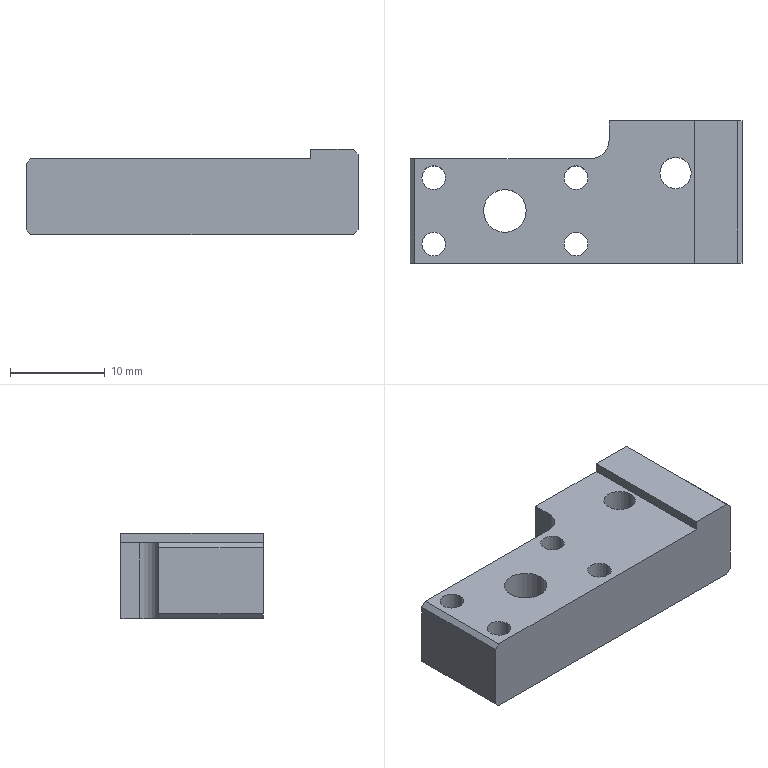Part | STEP file | FBDS-CS-035 | 1 solid | 30 faces | box 35 x 15 x 9 mm | volume 3093 mm3 | cylinder 15 | plane 15 | commonest cylinder face diameters 2.5 x8 3.3 x2 4.5 x2 8 x2 4 x1
STEP:
#1=CARTESIAN_POINT('',(26.35,-1.5,8.));
#2=VERTEX_POINT('',#1);
#3=CARTESIAN_POINT('',(29.65,-1.5,8.));
#4=VERTEX_POINT('',#3);
#5=CARTESIAN_POINT('',(28.,-1.5,8.));
#6=DIRECTION('',(0.,0.,1.));
#7=DIRECTION('',(1.,0.,0.));
#8=AXIS2_PLACEMENT_3D('',#5,#6,#7);
#9=CIRCLE('',#8,1.65);
#10=EDGE_CURVE('',#2,#4,#9,.T.);
#11=ORIENTED_EDGE('',*,*,#10,.T.);
#12=CARTESIAN_POINT('',(29.65,-1.5,0.));
#13=VERTEX_POINT('',#12);
#14=CARTESIAN_POINT('',(29.65,-1.5,0.));
#15=DIRECTION('',(0.,0.,-1.));
#16=VECTOR('',#15,1000.);
#17=LINE('',#14,#16);
#18=EDGE_CURVE('',#4,#13,#17,.T.);
#19=ORIENTED_EDGE('',*,*,#18,.T.);
#20=CARTESIAN_POINT('',(26.35,-1.5,0.));
#21=VERTEX_POINT('',#20);
#22=CARTESIAN_POINT('',(28.,-1.5,0.));
#23=DIRECTION('',(0.,0.,-1.));
#24=DIRECTION('',(-1.,0.,0.));
#25=AXIS2_PLACEMENT_3D('',#22,#23,#24);
#26=CIRCLE('',#25,1.65);
#27=EDGE_CURVE('',#13,#21,#26,.T.);
#28=ORIENTED_EDGE('',*,*,#27,.T.);
#29=CARTESIAN_POINT('',(26.35,-1.5,0.));
#30=DIRECTION('',(0.,0.,-1.));
#31=VECTOR('',#30,1000.);
#32=LINE('',#29,#31);
#33=EDGE_CURVE('',#2,#21,#32,.T.);
#34=ORIENTED_EDGE('',*,*,#33,.F.);
#35=EDGE_LOOP('',(#11,#19,#28,#34));
#36=FACE_OUTER_BOUND('',#35,.T.);
#37=CARTESIAN_POINT('',(28.,-1.5,0.));
#38=DIRECTION('',(0.,0.,-1.));
#39=DIRECTION('',(-1.,0.,0.));
#40=AXIS2_PLACEMENT_3D('',#37,#38,#39);
#41=CYLINDRICAL_SURFACE('',#40,1.65);
#42=ADVANCED_FACE('',(#36),#41,.F.);
#43=CARTESIAN_POINT('',(14.,-5.5,4.6));
#44=VERTEX_POINT('',#43);
#45=CARTESIAN_POINT('',(6.,-5.5,4.6));
#46=VERTEX_POINT('',#45);
#47=CARTESIAN_POINT('',(10.,-5.5,4.6));
#48=DIRECTION('',(0.,0.,-1.));
#49=DIRECTION('',(-1.,0.,0.));
#50=AXIS2_PLACEMENT_3D('',#47,#48,#49);
#51=CIRCLE('',#50,4.);
#52=EDGE_CURVE('',#44,#46,#51,.T.);
#53=ORIENTED_EDGE('',*,*,#52,.F.);
#54=CARTESIAN_POINT('',(14.,-5.5,0.));
#55=VERTEX_POINT('',#54);
#56=CARTESIAN_POINT('',(14.,-5.5,0.));
#57=DIRECTION('',(0.,0.,-1.));
#58=VECTOR('',#57,1000.);
#59=LINE('',#56,#58);
#60=EDGE_CURVE('',#44,#55,#59,.T.);
#61=ORIENTED_EDGE('',*,*,#60,.T.);
#62=CARTESIAN_POINT('',(6.,-5.5,0.));
#63=VERTEX_POINT('',#62);
#64=CARTESIAN_POINT('',(10.,-5.5,0.));
#65=DIRECTION('',(0.,0.,-1.));
#66=DIRECTION('',(-1.,0.,0.));
#67=AXIS2_PLACEMENT_3D('',#64,#65,#66);
#68=CIRCLE('',#67,4.);
#69=EDGE_CURVE('',#55,#63,#68,.T.);
#70=ORIENTED_EDGE('',*,*,#69,.T.);
#71=CARTESIAN_POINT('',(6.,-5.5,0.));
#72=DIRECTION('',(0.,0.,-1.));
#73=VECTOR('',#72,1000.);
#74=LINE('',#71,#73);
#75=EDGE_CURVE('',#46,#63,#74,.T.);
#76=ORIENTED_EDGE('',*,*,#75,.F.);
#77=EDGE_LOOP('',(#53,#61,#70,#76));
#78=FACE_OUTER_BOUND('',#77,.T.);
#79=CARTESIAN_POINT('',(10.,-5.5,0.));
#80=DIRECTION('',(0.,0.,-1.));
#81=DIRECTION('',(-1.,0.,0.));
#82=AXIS2_PLACEMENT_3D('',#79,#80,#81);
#83=CYLINDRICAL_SURFACE('',#82,4.);
#84=ADVANCED_FACE('',(#78),#83,.F.);
#85=CARTESIAN_POINT('',(7.75,-5.5,8.));
#86=VERTEX_POINT('',#85);
#87=CARTESIAN_POINT('',(12.25,-5.5,8.));
#88=VERTEX_POINT('',#87);
#89=CARTESIAN_POINT('',(10.,-5.5,8.));
#90=DIRECTION('',(0.,0.,1.));
#91=DIRECTION('',(1.,0.,0.));
#92=AXIS2_PLACEMENT_3D('',#89,#90,#91);
#93=CIRCLE('',#92,2.25);
#94=EDGE_CURVE('',#86,#88,#93,.T.);
#95=ORIENTED_EDGE('',*,*,#94,.T.);
#96=CARTESIAN_POINT('',(12.25,-5.5,4.6));
#97=VERTEX_POINT('',#96);
#98=CARTESIAN_POINT('',(12.25,-5.5,0.));
#99=DIRECTION('',(0.,0.,-1.));
#100=VECTOR('',#99,1000.);
#101=LINE('',#98,#100);
#102=EDGE_CURVE('',#88,#97,#101,.T.);
#103=ORIENTED_EDGE('',*,*,#102,.T.);
#104=CARTESIAN_POINT('',(7.75,-5.5,4.6));
#105=VERTEX_POINT('',#104);
#106=CARTESIAN_POINT('',(10.,-5.5,4.6));
#107=DIRECTION('',(0.,0.,-1.));
#108=DIRECTION('',(-1.,0.,0.));
#109=AXIS2_PLACEMENT_3D('',#106,#107,#108);
#110=CIRCLE('',#109,2.25);
#111=EDGE_CURVE('',#97,#105,#110,.T.);
#112=ORIENTED_EDGE('',*,*,#111,.T.);
#113=CARTESIAN_POINT('',(7.75,-5.5,0.));
#114=DIRECTION('',(0.,0.,-1.));
#115=VECTOR('',#114,1000.);
#116=LINE('',#113,#115);
#117=EDGE_CURVE('',#86,#105,#116,.T.);
#118=ORIENTED_EDGE('',*,*,#117,.F.);
#119=EDGE_LOOP('',(#95,#103,#112,#118));
#120=FACE_OUTER_BOUND('',#119,.T.);
#121=CARTESIAN_POINT('',(10.,-5.5,0.));
#122=DIRECTION('',(0.,0.,-1.));
#123=DIRECTION('',(-1.,0.,0.));
#124=AXIS2_PLACEMENT_3D('',#121,#122,#123);
#125=CYLINDRICAL_SURFACE('',#124,2.25);
#126=ADVANCED_FACE('',(#120),#125,.F.);
#127=CARTESIAN_POINT('',(16.25,-2.,8.));
#128=VERTEX_POINT('',#127);
#129=CARTESIAN_POINT('',(18.75,-2.,8.));
#130=VERTEX_POINT('',#129);
#131=CARTESIAN_POINT('',(17.5,-2.,8.));
#132=DIRECTION('',(0.,0.,1.));
#133=DIRECTION('',(1.,0.,0.));
#134=AXIS2_PLACEMENT_3D('',#131,#132,#133);
#135=CIRCLE('',#134,1.25);
#136=EDGE_CURVE('',#128,#130,#135,.T.);
#137=ORIENTED_EDGE('',*,*,#136,.T.);
#138=CARTESIAN_POINT('',(18.75,-2.,0.));
#139=VERTEX_POINT('',#138);
#140=CARTESIAN_POINT('',(18.75,-2.,0.));
#141=DIRECTION('',(0.,0.,-1.));
#142=VECTOR('',#141,1000.);
#143=LINE('',#140,#142);
#144=EDGE_CURVE('',#130,#139,#143,.T.);
#145=ORIENTED_EDGE('',*,*,#144,.T.);
#146=CARTESIAN_POINT('',(16.25,-2.,0.));
#147=VERTEX_POINT('',#146);
#148=CARTESIAN_POINT('',(17.5,-2.,0.));
#149=DIRECTION('',(0.,0.,-1.));
#150=DIRECTION('',(-1.,0.,0.));
#151=AXIS2_PLACEMENT_3D('',#148,#149,#150);
#152=CIRCLE('',#151,1.25);
#153=EDGE_CURVE('',#139,#147,#152,.T.);
#154=ORIENTED_EDGE('',*,*,#153,.T.);
#155=CARTESIAN_POINT('',(16.25,-2.,0.));
#156=DIRECTION('',(0.,0.,-1.));
#157=VECTOR('',#156,1000.);
#158=LINE('',#155,#157);
#159=EDGE_CURVE('',#128,#147,#158,.T.);
#160=ORIENTED_EDGE('',*,*,#159,.F.);
#161=EDGE_LOOP('',(#137,#145,#154,#160));
#162=FACE_OUTER_BOUND('',#161,.T.);
#163=CARTESIAN_POINT('',(17.5,-2.,0.));
#164=DIRECTION('',(0.,0.,-1.));
#165=DIRECTION('',(-1.,0.,0.));
#166=AXIS2_PLACEMENT_3D('',#163,#164,#165);
#167=CYLINDRICAL_SURFACE('',#166,1.25);
#168=ADVANCED_FACE('',(#162),#167,.F.);
#169=CARTESIAN_POINT('',(16.25,-9.,8.));
#170=VERTEX_POINT('',#169);
#171=CARTESIAN_POINT('',(18.75,-9.,8.));
#172=VERTEX_POINT('',#171);
#173=CARTESIAN_POINT('',(17.5,-9.,8.));
#174=DIRECTION('',(0.,0.,1.));
#175=DIRECTION('',(1.,0.,0.));
#176=AXIS2_PLACEMENT_3D('',#173,#174,#175);
#177=CIRCLE('',#176,1.25);
#178=EDGE_CURVE('',#170,#172,#177,.T.);
#179=ORIENTED_EDGE('',*,*,#178,.T.);
#180=CARTESIAN_POINT('',(18.75,-9.,0.));
#181=VERTEX_POINT('',#180);
#182=CARTESIAN_POINT('',(18.75,-9.,0.));
#183=DIRECTION('',(0.,0.,-1.));
#184=VECTOR('',#183,1000.);
#185=LINE('',#182,#184);
#186=EDGE_CURVE('',#172,#181,#185,.T.);
#187=ORIENTED_EDGE('',*,*,#186,.T.);
#188=CARTESIAN_POINT('',(16.25,-9.,0.));
#189=VERTEX_POINT('',#188);
#190=CARTESIAN_POINT('',(17.5,-9.,0.));
#191=DIRECTION('',(0.,0.,-1.));
#192=DIRECTION('',(-1.,0.,0.));
#193=AXIS2_PLACEMENT_3D('',#190,#191,#192);
#194=CIRCLE('',#193,1.25);
#195=EDGE_CURVE('',#181,#189,#194,.T.);
#196=ORIENTED_EDGE('',*,*,#195,.T.);
#197=CARTESIAN_POINT('',(16.25,-9.,0.));
#198=DIRECTION('',(0.,0.,-1.));
#199=VECTOR('',#198,1000.);
#200=LINE('',#197,#199);
#201=EDGE_CURVE('',#170,#189,#200,.T.);
#202=ORIENTED_EDGE('',*,*,#201,.F.);
#203=EDGE_LOOP('',(#179,#187,#196,#202));
#204=FACE_OUTER_BOUND('',#203,.T.);
#205=CARTESIAN_POINT('',(17.5,-9.,0.));
#206=DIRECTION('',(0.,0.,-1.));
#207=DIRECTION('',(-1.,0.,0.));
#208=AXIS2_PLACEMENT_3D('',#205,#206,#207);
#209=CYLINDRICAL_SURFACE('',#208,1.25);
#210=ADVANCED_FACE('',(#204),#209,.F.);
#211=CARTESIAN_POINT('',(1.25,-9.,8.));
#212=VERTEX_POINT('',#211);
#213=CARTESIAN_POINT('',(3.75,-9.,8.));
#214=VERTEX_POINT('',#213);
#215=CARTESIAN_POINT('',(2.5,-9.,8.));
#216=DIRECTION('',(0.,0.,1.));
#217=DIRECTION('',(1.,0.,0.));
#218=AXIS2_PLACEMENT_3D('',#215,#216,#217);
#219=CIRCLE('',#218,1.25);
#220=EDGE_CURVE('',#212,#214,#219,.T.);
#221=ORIENTED_EDGE('',*,*,#220,.T.);
#222=CARTESIAN_POINT('',(3.75,-9.,0.));
#223=VERTEX_POINT('',#222);
#224=CARTESIAN_POINT('',(3.75,-9.,0.));
#225=DIRECTION('',(0.,0.,-1.));
#226=VECTOR('',#225,1000.);
#227=LINE('',#224,#226);
#228=EDGE_CURVE('',#214,#223,#227,.T.);
#229=ORIENTED_EDGE('',*,*,#228,.T.);
#230=CARTESIAN_POINT('',(1.25,-9.,0.));
#231=VERTEX_POINT('',#230);
#232=CARTESIAN_POINT('',(2.5,-9.,0.));
#233=DIRECTION('',(0.,0.,-1.));
#234=DIRECTION('',(-1.,0.,0.));
#235=AXIS2_PLACEMENT_3D('',#232,#233,#234);
#236=CIRCLE('',#235,1.25);
#237=EDGE_CURVE('',#223,#231,#236,.T.);
#238=ORIENTED_EDGE('',*,*,#237,.T.);
#239=CARTESIAN_POINT('',(1.25,-9.,0.));
#240=DIRECTION('',(0.,0.,-1.));
#241=VECTOR('',#240,1000.);
#242=LINE('',#239,#241);
#243=EDGE_CURVE('',#212,#231,#242,.T.);
#244=ORIENTED_EDGE('',*,*,#243,.F.);
#245=EDGE_LOOP('',(#221,#229,#238,#244));
#246=FACE_OUTER_BOUND('',#245,.T.);
#247=CARTESIAN_POINT('',(2.5,-9.,0.));
#248=DIRECTION('',(0.,0.,-1.));
#249=DIRECTION('',(-1.,0.,0.));
#250=AXIS2_PLACEMENT_3D('',#247,#248,#249);
#251=CYLINDRICAL_SURFACE('',#250,1.25);
#252=ADVANCED_FACE('',(#246),#251,.F.);
#253=CARTESIAN_POINT('',(1.25,-2.,8.));
#254=VERTEX_POINT('',#253);
#255=CARTESIAN_POINT('',(3.75,-2.,8.));
#256=VERTEX_POINT('',#255);
#257=CARTESIAN_POINT('',(2.5,-2.,8.));
#258=DIRECTION('',(0.,0.,1.));
#259=DIRECTION('',(1.,0.,0.));
#260=AXIS2_PLACEMENT_3D('',#257,#258,#259);
#261=CIRCLE('',#260,1.25);
#262=EDGE_CURVE('',#254,#256,#261,.T.);
#263=ORIENTED_EDGE('',*,*,#262,.T.);
#264=CARTESIAN_POINT('',(3.75,-2.,0.));
#265=VERTEX_POINT('',#264);
#266=CARTESIAN_POINT('',(3.75,-2.,0.));
#267=DIRECTION('',(0.,0.,-1.));
#268=VECTOR('',#267,1000.);
#269=LINE('',#266,#268);
#270=EDGE_CURVE('',#256,#265,#269,.T.);
#271=ORIENTED_EDGE('',*,*,#270,.T.);
#272=CARTESIAN_POINT('',(1.25,-2.,0.));
#273=VERTEX_POINT('',#272);
#274=CARTESIAN_POINT('',(2.5,-2.,0.));
#275=DIRECTION('',(0.,0.,-1.));
#276=DIRECTION('',(-1.,0.,0.));
#277=AXIS2_PLACEMENT_3D('',#274,#275,#276);
#278=CIRCLE('',#277,1.25);
#279=EDGE_CURVE('',#265,#273,#278,.T.);
#280=ORIENTED_EDGE('',*,*,#279,.T.);
#281=CARTESIAN_POINT('',(1.25,-2.,0.));
#282=DIRECTION('',(0.,0.,-1.));
#283=VECTOR('',#282,1000.);
#284=LINE('',#281,#283);
#285=EDGE_CURVE('',#254,#273,#284,.T.);
#286=ORIENTED_EDGE('',*,*,#285,.F.);
#287=EDGE_LOOP('',(#263,#271,#280,#286));
#288=FACE_OUTER_BOUND('',#287,.T.);
#289=CARTESIAN_POINT('',(2.5,-2.,0.));
#290=DIRECTION('',(0.,0.,-1.));
#291=DIRECTION('',(-1.,0.,0.));
#292=AXIS2_PLACEMENT_3D('',#289,#290,#291);
#293=CYLINDRICAL_SURFACE('',#292,1.25);
#294=ADVANCED_FACE('',(#288),#293,.F.);
#295=CARTESIAN_POINT('',(19.,0.,8.));
#296=VERTEX_POINT('',#295);
#297=CARTESIAN_POINT('',(0.5,0.,8.));
#298=VERTEX_POINT('',#297);
#299=CARTESIAN_POINT('',(0.,0.,8.));
#300=DIRECTION('',(-1.,0.,0.));
#301=VECTOR('',#300,1000.);
#302=LINE('',#299,#301);
#303=EDGE_CURVE('',#296,#298,#302,.T.);
#304=ORIENTED_EDGE('',*,*,#303,.F.);
#305=CARTESIAN_POINT('',(19.,0.,0.));
#306=VERTEX_POINT('',#305);
#307=CARTESIAN_POINT('',(19.,0.,0.));
#308=DIRECTION('',(0.,0.,-1.));
#309=VECTOR('',#308,1000.);
#310=LINE('',#307,#309);
#311=EDGE_CURVE('',#296,#306,#310,.T.);
#312=ORIENTED_EDGE('',*,*,#311,.T.);
#313=CARTESIAN_POINT('',(0.5,0.,0.));
#314=VERTEX_POINT('',#313);
#315=CARTESIAN_POINT('',(0.,0.,0.));
#316=DIRECTION('',(-1.,0.,0.));
#317=VECTOR('',#316,1000.);
#318=LINE('',#315,#317);
#319=EDGE_CURVE('',#306,#314,#318,.T.);
#320=ORIENTED_EDGE('',*,*,#319,.T.);
#321=CARTESIAN_POINT('',(0.,0.,0.5));
#322=VERTEX_POINT('',#321);
#323=CARTESIAN_POINT('',(0.,0.,0.5));
#324=DIRECTION('',(-0.7071,0.,0.7071));
#325=VECTOR('',#324,1000.);
#326=LINE('',#323,#325);
#327=EDGE_CURVE('',#314,#322,#326,.T.);
#328=ORIENTED_EDGE('',*,*,#327,.T.);
#329=CARTESIAN_POINT('',(0.,0.,7.5));
#330=VERTEX_POINT('',#329);
#331=CARTESIAN_POINT('',(0.,0.,8.));
#332=DIRECTION('',(0.,0.,-1.));
#333=VECTOR('',#332,1000.);
#334=LINE('',#331,#333);
#335=EDGE_CURVE('',#330,#322,#334,.T.);
#336=ORIENTED_EDGE('',*,*,#335,.F.);
#337=CARTESIAN_POINT('',(0.5,0.,8.));
#338=DIRECTION('',(0.7071,0.,0.7071));
#339=VECTOR('',#338,1000.);
#340=LINE('',#337,#339);
#341=EDGE_CURVE('',#330,#298,#340,.T.);
#342=ORIENTED_EDGE('',*,*,#341,.T.);
#343=EDGE_LOOP('',(#304,#312,#320,#328,#336,#342));
#344=FACE_OUTER_BOUND('',#343,.T.);
#345=CARTESIAN_POINT('',(0.,0.,8.));
#346=DIRECTION('',(0.,-1.,0.));
#347=DIRECTION('',(0.,0.,-1.));
#348=AXIS2_PLACEMENT_3D('',#345,#346,#347);
#349=PLANE('',#348);
#350=ADVANCED_FACE('',(#344),#349,.F.);
#351=ORIENTED_EDGE('',*,*,#335,.T.);
#352=CARTESIAN_POINT('',(0.,-11.,0.5));
#353=VERTEX_POINT('',#352);
#354=CARTESIAN_POINT('',(0.,0.,0.5));
#355=DIRECTION('',(0.,-1.,0.));
#356=VECTOR('',#355,1000.);
#357=LINE('',#354,#356);
#358=EDGE_CURVE('',#322,#353,#357,.T.);
#359=ORIENTED_EDGE('',*,*,#358,.T.);
#360=CARTESIAN_POINT('',(0.,-11.,7.5));
#361=VERTEX_POINT('',#360);
#362=CARTESIAN_POINT('',(0.,-11.,8.));
#363=DIRECTION('',(0.,0.,-1.));
#364=VECTOR('',#363,1000.);
#365=LINE('',#362,#364);
#366=EDGE_CURVE('',#361,#353,#365,.T.);
#367=ORIENTED_EDGE('',*,*,#366,.F.);
#368=CARTESIAN_POINT('',(0.,0.,7.5));
#369=DIRECTION('',(0.,1.,0.));
#370=VECTOR('',#369,1000.);
#371=LINE('',#368,#370);
#372=EDGE_CURVE('',#361,#330,#371,.T.);
#373=ORIENTED_EDGE('',*,*,#372,.T.);
#374=EDGE_LOOP('',(#351,#359,#367,#373));
#375=FACE_OUTER_BOUND('',#374,.T.);
#376=CARTESIAN_POINT('',(0.,0.,8.));
#377=DIRECTION('',(1.,0.,0.));
#378=DIRECTION('',(0.,0.,-1.));
#379=AXIS2_PLACEMENT_3D('',#376,#377,#378);
#380=PLANE('',#379);
#381=ADVANCED_FACE('',(#375),#380,.F.);
#382=CARTESIAN_POINT('',(35.,-11.,8.5));
#383=VERTEX_POINT('',#382);
#384=CARTESIAN_POINT('',(35.,-11.,0.5));
#385=VERTEX_POINT('',#384);
#386=CARTESIAN_POINT('',(35.,-11.,8.));
#387=DIRECTION('',(0.,0.,-1.));
#388=VECTOR('',#387,1000.);
#389=LINE('',#386,#388);
#390=EDGE_CURVE('',#383,#385,#389,.T.);
#391=ORIENTED_EDGE('',*,*,#390,.F.);
#392=CARTESIAN_POINT('',(34.5,-11.,9.));
#393=VERTEX_POINT('',#392);
#394=CARTESIAN_POINT('',(34.5,-11.,9.));
#395=DIRECTION('',(-0.7071,0.,0.7071));
#396=VECTOR('',#395,1000.);
#397=LINE('',#394,#396);
#398=EDGE_CURVE('',#383,#393,#397,.T.);
#399=ORIENTED_EDGE('',*,*,#398,.T.);
#400=CARTESIAN_POINT('',(30.,-11.,9.));
#401=VERTEX_POINT('',#400);
#402=CARTESIAN_POINT('',(35.,-11.,9.));
#403=DIRECTION('',(1.,0.,0.));
#404=VECTOR('',#403,1000.);
#405=LINE('',#402,#404);
#406=EDGE_CURVE('',#401,#393,#405,.T.);
#407=ORIENTED_EDGE('',*,*,#406,.F.);
#408=CARTESIAN_POINT('',(30.,-11.,8.));
#409=VERTEX_POINT('',#408);
#410=CARTESIAN_POINT('',(30.,-11.,9.));
#411=DIRECTION('',(0.,0.,-1.));
#412=VECTOR('',#411,1000.);
#413=LINE('',#410,#412);
#414=EDGE_CURVE('',#401,#409,#413,.T.);
#415=ORIENTED_EDGE('',*,*,#414,.T.);
#416=CARTESIAN_POINT('',(0.5,-11.,8.));
#417=VERTEX_POINT('',#416);
#418=CARTESIAN_POINT('',(0.,-11.,8.));
#419=DIRECTION('',(1.,0.,0.));
#420=VECTOR('',#419,1000.);
#421=LINE('',#418,#420);
#422=EDGE_CURVE('',#417,#409,#421,.T.);
#423=ORIENTED_EDGE('',*,*,#422,.F.);
#424=CARTESIAN_POINT('',(0.5,-11.,8.));
#425=DIRECTION('',(-0.7071,0.,-0.7071));
#426=VECTOR('',#425,1000.);
#427=LINE('',#424,#426);
#428=EDGE_CURVE('',#417,#361,#427,.T.);
#429=ORIENTED_EDGE('',*,*,#428,.T.);
#430=ORIENTED_EDGE('',*,*,#366,.T.);
#431=CARTESIAN_POINT('',(0.5,-11.,0.));
#432=VERTEX_POINT('',#431);
#433=CARTESIAN_POINT('',(0.,-11.,0.5));
#434=DIRECTION('',(0.7071,0.,-0.7071));
#435=VECTOR('',#434,1000.);
#436=LINE('',#433,#435);
#437=EDGE_CURVE('',#353,#432,#436,.T.);
#438=ORIENTED_EDGE('',*,*,#437,.T.);
#439=CARTESIAN_POINT('',(34.5,-11.,0.));
#440=VERTEX_POINT('',#439);
#441=CARTESIAN_POINT('',(0.,-11.,0.));
#442=DIRECTION('',(1.,0.,0.));
#443=VECTOR('',#442,1000.);
#444=LINE('',#441,#443);
#445=EDGE_CURVE('',#432,#440,#444,.T.);
#446=ORIENTED_EDGE('',*,*,#445,.T.);
#447=CARTESIAN_POINT('',(35.,-11.,0.5));
#448=DIRECTION('',(0.7071,0.,0.7071));
#449=VECTOR('',#448,1000.);
#450=LINE('',#447,#449);
#451=EDGE_CURVE('',#440,#385,#450,.T.);
#452=ORIENTED_EDGE('',*,*,#451,.T.);
#453=EDGE_LOOP('',(#391,#399,#407,#415,#423,#429,#430,#438,#446,#452));
#454=FACE_OUTER_BOUND('',#453,.T.);
#455=CARTESIAN_POINT('',(0.,-11.,8.));
#456=DIRECTION('',(0.,1.,0.));
#457=DIRECTION('',(0.,0.,1.));
#458=AXIS2_PLACEMENT_3D('',#455,#456,#457);
#459=PLANE('',#458);
#460=ADVANCED_FACE('',(#454),#459,.F.);
#461=CARTESIAN_POINT('',(35.,4.,0.5));
#462=VERTEX_POINT('',#461);
#463=CARTESIAN_POINT('',(35.,0.,0.5));
#464=DIRECTION('',(0.,1.,0.));
#465=VECTOR('',#464,1000.);
#466=LINE('',#463,#465);
#467=EDGE_CURVE('',#385,#462,#466,.T.);
#468=ORIENTED_EDGE('',*,*,#467,.T.);
#469=CARTESIAN_POINT('',(35.,4.,8.5));
#470=VERTEX_POINT('',#469);
#471=CARTESIAN_POINT('',(35.,4.,8.5));
#472=DIRECTION('',(0.,0.,-1.));
#473=VECTOR('',#472,1000.);
#474=LINE('',#471,#473);
#475=EDGE_CURVE('',#470,#462,#474,.T.);
#476=ORIENTED_EDGE('',*,*,#475,.F.);
#477=CARTESIAN_POINT('',(35.,0.,8.5));
#478=DIRECTION('',(0.,-1.,0.));
#479=VECTOR('',#478,1000.);
#480=LINE('',#477,#479);
#481=EDGE_CURVE('',#470,#383,#480,.T.);
#482=ORIENTED_EDGE('',*,*,#481,.T.);
#483=ORIENTED_EDGE('',*,*,#390,.T.);
#484=EDGE_LOOP('',(#468,#476,#482,#483));
#485=FACE_OUTER_BOUND('',#484,.T.);
#486=CARTESIAN_POINT('',(35.,0.,8.));
#487=DIRECTION('',(-1.,0.,0.));
#488=DIRECTION('',(0.,0.,1.));
#489=AXIS2_PLACEMENT_3D('',#486,#487,#488);
#490=PLANE('',#489);
#491=ADVANCED_FACE('',(#485),#490,.F.);
#492=ORIENTED_EDGE('',*,*,#10,.F.);
#493=CARTESIAN_POINT('',(28.,-1.5,8.));
#494=DIRECTION('',(0.,0.,1.));
#495=DIRECTION('',(1.,0.,0.));
#496=AXIS2_PLACEMENT_3D('',#493,#494,#495);
#497=CIRCLE('',#496,1.65);
#498=EDGE_CURVE('',#4,#2,#497,.T.);
#499=ORIENTED_EDGE('',*,*,#498,.F.);
#500=EDGE_LOOP('',(#492,#499));
#501=FACE_BOUND('',#500,.T.);
#502=CARTESIAN_POINT('',(30.,4.,8.));
#503=VERTEX_POINT('',#502);
#504=CARTESIAN_POINT('',(30.,0.,8.));
#505=DIRECTION('',(0.,-1.,0.));
#506=VECTOR('',#505,1000.);
#507=LINE('',#504,#506);
#508=EDGE_CURVE('',#503,#409,#507,.T.);
#509=ORIENTED_EDGE('',*,*,#508,.F.);
#510=CARTESIAN_POINT('',(21.,4.,8.));
#511=VERTEX_POINT('',#510);
#512=CARTESIAN_POINT('',(21.,4.,8.));
#513=DIRECTION('',(1.,0.,0.));
#514=VECTOR('',#513,1000.);
#515=LINE('',#512,#514);
#516=EDGE_CURVE('',#511,#503,#515,.T.);
#517=ORIENTED_EDGE('',*,*,#516,.F.);
#518=CARTESIAN_POINT('',(21.,2.,8.));
#519=VERTEX_POINT('',#518);
#520=CARTESIAN_POINT('',(21.,4.,8.));
#521=DIRECTION('',(0.,-1.,0.));
#522=VECTOR('',#521,1000.);
#523=LINE('',#520,#522);
#524=EDGE_CURVE('',#511,#519,#523,.T.);
#525=ORIENTED_EDGE('',*,*,#524,.T.);
#526=CARTESIAN_POINT('',(19.,2.,8.));
#527=DIRECTION('',(0.,0.,-1.));
#528=DIRECTION('',(1.,0.,0.));
#529=AXIS2_PLACEMENT_3D('',#526,#527,#528);
#530=CIRCLE('',#529,2.);
#531=EDGE_CURVE('',#519,#296,#530,.T.);
#532=ORIENTED_EDGE('',*,*,#531,.T.);
#533=ORIENTED_EDGE('',*,*,#303,.T.);
#534=CARTESIAN_POINT('',(0.5,-11.,8.));
#535=DIRECTION('',(0.,-1.,0.));
#536=VECTOR('',#535,1000.);
#537=LINE('',#534,#536);
#538=EDGE_CURVE('',#298,#417,#537,.T.);
#539=ORIENTED_EDGE('',*,*,#538,.T.);
#540=ORIENTED_EDGE('',*,*,#422,.T.);
#541=EDGE_LOOP('',(#509,#517,#525,#532,#533,#539,#540));
#542=FACE_OUTER_BOUND('',#541,.T.);
#543=ORIENTED_EDGE('',*,*,#94,.F.);
#544=CARTESIAN_POINT('',(10.,-5.5,8.));
#545=DIRECTION('',(0.,0.,1.));
#546=DIRECTION('',(1.,0.,0.));
#547=AXIS2_PLACEMENT_3D('',#544,#545,#546);
#548=CIRCLE('',#547,2.25);
#549=EDGE_CURVE('',#88,#86,#548,.T.);
#550=ORIENTED_EDGE('',*,*,#549,.F.);
#551=EDGE_LOOP('',(#543,#550));
#552=FACE_BOUND('',#551,.T.);
#553=ORIENTED_EDGE('',*,*,#136,.F.);
#554=CARTESIAN_POINT('',(17.5,-2.,8.));
#555=DIRECTION('',(0.,0.,1.));
#556=DIRECTION('',(1.,0.,0.));
#557=AXIS2_PLACEMENT_3D('',#554,#555,#556);
#558=CIRCLE('',#557,1.25);
#559=EDGE_CURVE('',#130,#128,#558,.T.);
#560=ORIENTED_EDGE('',*,*,#559,.F.);
#561=EDGE_LOOP('',(#553,#560));
#562=FACE_BOUND('',#561,.T.);
#563=ORIENTED_EDGE('',*,*,#178,.F.);
#564=CARTESIAN_POINT('',(17.5,-9.,8.));
#565=DIRECTION('',(0.,0.,1.));
#566=DIRECTION('',(1.,0.,0.));
#567=AXIS2_PLACEMENT_3D('',#564,#565,#566);
#568=CIRCLE('',#567,1.25);
#569=EDGE_CURVE('',#172,#170,#568,.T.);
#570=ORIENTED_EDGE('',*,*,#569,.F.);
#571=EDGE_LOOP('',(#563,#570));
#572=FACE_BOUND('',#571,.T.);
#573=ORIENTED_EDGE('',*,*,#220,.F.);
#574=CARTESIAN_POINT('',(2.5,-9.,8.));
#575=DIRECTION('',(0.,0.,1.));
#576=DIRECTION('',(1.,0.,0.));
#577=AXIS2_PLACEMENT_3D('',#574,#575,#576);
#578=CIRCLE('',#577,1.25);
#579=EDGE_CURVE('',#214,#212,#578,.T.);
#580=ORIENTED_EDGE('',*,*,#579,.F.);
#581=EDGE_LOOP('',(#573,#580));
#582=FACE_BOUND('',#581,.T.);
#583=ORIENTED_EDGE('',*,*,#262,.F.);
#584=CARTESIAN_POINT('',(2.5,-2.,8.));
#585=DIRECTION('',(0.,0.,1.));
#586=DIRECTION('',(1.,0.,0.));
#587=AXIS2_PLACEMENT_3D('',#584,#585,#586);
#588=CIRCLE('',#587,1.25);
#589=EDGE_CURVE('',#256,#254,#588,.T.);
#590=ORIENTED_EDGE('',*,*,#589,.F.);
#591=EDGE_LOOP('',(#583,#590));
#592=FACE_BOUND('',#591,.T.);
#593=CARTESIAN_POINT('',(0.,0.,8.));
#594=DIRECTION('',(0.,0.,1.));
#595=DIRECTION('',(1.,0.,0.));
#596=AXIS2_PLACEMENT_3D('',#593,#594,#595);
#597=PLANE('',#596);
#598=ADVANCED_FACE('',(#501,#542,#552,#562,#572,#582,#592),#597,.T.);
#599=CARTESIAN_POINT('',(28.,-1.5,0.));
#600=DIRECTION('',(0.,0.,-1.));
#601=DIRECTION('',(-1.,0.,0.));
#602=AXIS2_PLACEMENT_3D('',#599,#600,#601);
#603=CIRCLE('',#602,1.65);
#604=EDGE_CURVE('',#21,#13,#603,.T.);
#605=ORIENTED_EDGE('',*,*,#604,.F.);
#606=ORIENTED_EDGE('',*,*,#27,.F.);
#607=EDGE_LOOP('',(#605,#606));
#608=FACE_BOUND('',#607,.T.);
#609=CARTESIAN_POINT('',(10.,-5.5,0.));
#610=DIRECTION('',(0.,0.,-1.));
#611=DIRECTION('',(-1.,0.,0.));
#612=AXIS2_PLACEMENT_3D('',#609,#610,#611);
#613=CIRCLE('',#612,4.);
#614=EDGE_CURVE('',#63,#55,#613,.T.);
#615=ORIENTED_EDGE('',*,*,#614,.F.);
#616=ORIENTED_EDGE('',*,*,#69,.F.);
#617=EDGE_LOOP('',(#615,#616));
#618=FACE_BOUND('',#617,.T.);
#619=CARTESIAN_POINT('',(17.5,-2.,0.));
#620=DIRECTION('',(0.,0.,-1.));
#621=DIRECTION('',(-1.,0.,0.));
#622=AXIS2_PLACEMENT_3D('',#619,#620,#621);
#623=CIRCLE('',#622,1.25);
#624=EDGE_CURVE('',#147,#139,#623,.T.);
#625=ORIENTED_EDGE('',*,*,#624,.F.);
#626=ORIENTED_EDGE('',*,*,#153,.F.);
#627=EDGE_LOOP('',(#625,#626));
#628=FACE_BOUND('',#627,.T.);
#629=CARTESIAN_POINT('',(17.5,-9.,0.));
#630=DIRECTION('',(0.,0.,-1.));
#631=DIRECTION('',(-1.,0.,0.));
#632=AXIS2_PLACEMENT_3D('',#629,#630,#631);
#633=CIRCLE('',#632,1.25);
#634=EDGE_CURVE('',#189,#181,#633,.T.);
#635=ORIENTED_EDGE('',*,*,#634,.F.);
#636=ORIENTED_EDGE('',*,*,#195,.F.);
#637=EDGE_LOOP('',(#635,#636));
#638=FACE_BOUND('',#637,.T.);
#639=CARTESIAN_POINT('',(2.5,-9.,0.));
#640=DIRECTION('',(0.,0.,-1.));
#641=DIRECTION('',(-1.,0.,0.));
#642=AXIS2_PLACEMENT_3D('',#639,#640,#641);
#643=CIRCLE('',#642,1.25);
#644=EDGE_CURVE('',#231,#223,#643,.T.);
#645=ORIENTED_EDGE('',*,*,#644,.F.);
#646=ORIENTED_EDGE('',*,*,#237,.F.);
#647=EDGE_LOOP('',(#645,#646));
#648=FACE_BOUND('',#647,.T.);
#649=CARTESIAN_POINT('',(2.5,-2.,0.));
#650=DIRECTION('',(0.,0.,-1.));
#651=DIRECTION('',(-1.,0.,0.));
#652=AXIS2_PLACEMENT_3D('',#649,#650,#651);
#653=CIRCLE('',#652,1.25);
#654=EDGE_CURVE('',#273,#265,#653,.T.);
#655=ORIENTED_EDGE('',*,*,#654,.F.);
#656=ORIENTED_EDGE('',*,*,#279,.F.);
#657=EDGE_LOOP('',(#655,#656));
#658=FACE_BOUND('',#657,.T.);
#659=ORIENTED_EDGE('',*,*,#319,.F.);
#660=CARTESIAN_POINT('',(21.,2.,0.));
#661=VERTEX_POINT('',#660);
#662=CARTESIAN_POINT('',(19.,2.,0.));
#663=DIRECTION('',(0.,0.,1.));
#664=DIRECTION('',(1.,0.,0.));
#665=AXIS2_PLACEMENT_3D('',#662,#663,#664);
#666=CIRCLE('',#665,2.);
#667=EDGE_CURVE('',#306,#661,#666,.T.);
#668=ORIENTED_EDGE('',*,*,#667,.T.);
#669=CARTESIAN_POINT('',(21.,4.,0.));
#670=VERTEX_POINT('',#669);
#671=CARTESIAN_POINT('',(21.,4.,0.));
#672=DIRECTION('',(0.,-1.,0.));
#673=VECTOR('',#672,1000.);
#674=LINE('',#671,#673);
#675=EDGE_CURVE('',#670,#661,#674,.T.);
#676=ORIENTED_EDGE('',*,*,#675,.F.);
#677=CARTESIAN_POINT('',(34.5,4.,0.));
#678=VERTEX_POINT('',#677);
#679=CARTESIAN_POINT('',(34.5,4.,0.));
#680=DIRECTION('',(-1.,0.,0.));
#681=VECTOR('',#680,1000.);
#682=LINE('',#679,#681);
#683=EDGE_CURVE('',#678,#670,#682,.T.);
#684=ORIENTED_EDGE('',*,*,#683,.F.);
#685=CARTESIAN_POINT('',(34.5,0.,0.));
#686=DIRECTION('',(0.,-1.,0.));
#687=VECTOR('',#686,1000.);
#688=LINE('',#685,#687);
#689=EDGE_CURVE('',#678,#440,#688,.T.);
#690=ORIENTED_EDGE('',*,*,#689,.T.);
#691=ORIENTED_EDGE('',*,*,#445,.F.);
#692=CARTESIAN_POINT('',(0.5,0.,0.));
#693=DIRECTION('',(0.,1.,0.));
#694=VECTOR('',#693,1000.);
#695=LINE('',#692,#694);
#696=EDGE_CURVE('',#432,#314,#695,.T.);
#697=ORIENTED_EDGE('',*,*,#696,.T.);
#698=EDGE_LOOP('',(#659,#668,#676,#684,#690,#691,#697));
#699=FACE_OUTER_BOUND('',#698,.T.);
#700=CARTESIAN_POINT('',(0.,0.,0.));
#701=DIRECTION('',(0.,0.,1.));
#702=DIRECTION('',(1.,0.,0.));
#703=AXIS2_PLACEMENT_3D('',#700,#701,#702);
#704=PLANE('',#703);
#705=ADVANCED_FACE('',(#608,#618,#628,#638,#648,#658,#699),#704,.F.);
#706=ORIENTED_EDGE('',*,*,#270,.F.);
#707=ORIENTED_EDGE('',*,*,#589,.T.);
#708=ORIENTED_EDGE('',*,*,#285,.T.);
#709=ORIENTED_EDGE('',*,*,#654,.T.);
#710=EDGE_LOOP('',(#706,#707,#708,#709));
#711=FACE_OUTER_BOUND('',#710,.T.);
#712=CARTESIAN_POINT('',(2.5,-2.,0.));
#713=DIRECTION('',(0.,0.,-1.));
#714=DIRECTION('',(-1.,0.,0.));
#715=AXIS2_PLACEMENT_3D('',#712,#713,#714);
#716=CYLINDRICAL_SURFACE('',#715,1.25);
#717=ADVANCED_FACE('',(#711),#716,.F.);
#718=ORIENTED_EDGE('',*,*,#228,.F.);
#719=ORIENTED_EDGE('',*,*,#579,.T.);
#720=ORIENTED_EDGE('',*,*,#243,.T.);
#721=ORIENTED_EDGE('',*,*,#644,.T.);
#722=EDGE_LOOP('',(#718,#719,#720,#721));
#723=FACE_OUTER_BOUND('',#722,.T.);
#724=CARTESIAN_POINT('',(2.5,-9.,0.));
#725=DIRECTION('',(0.,0.,-1.));
#726=DIRECTION('',(-1.,0.,0.));
#727=AXIS2_PLACEMENT_3D('',#724,#725,#726);
#728=CYLINDRICAL_SURFACE('',#727,1.25);
#729=ADVANCED_FACE('',(#723),#728,.F.);
#730=ORIENTED_EDGE('',*,*,#186,.F.);
#731=ORIENTED_EDGE('',*,*,#569,.T.);
#732=ORIENTED_EDGE('',*,*,#201,.T.);
#733=ORIENTED_EDGE('',*,*,#634,.T.);
#734=EDGE_LOOP('',(#730,#731,#732,#733));
#735=FACE_OUTER_BOUND('',#734,.T.);
#736=CARTESIAN_POINT('',(17.5,-9.,0.));
#737=DIRECTION('',(0.,0.,-1.));
#738=DIRECTION('',(-1.,0.,0.));
#739=AXIS2_PLACEMENT_3D('',#736,#737,#738);
#740=CYLINDRICAL_SURFACE('',#739,1.25);
#741=ADVANCED_FACE('',(#735),#740,.F.);
#742=ORIENTED_EDGE('',*,*,#144,.F.);
#743=ORIENTED_EDGE('',*,*,#559,.T.);
#744=ORIENTED_EDGE('',*,*,#159,.T.);
#745=ORIENTED_EDGE('',*,*,#624,.T.);
#746=EDGE_LOOP('',(#742,#743,#744,#745));
#747=FACE_OUTER_BOUND('',#746,.T.);
#748=CARTESIAN_POINT('',(17.5,-2.,0.));
#749=DIRECTION('',(0.,0.,-1.));
#750=DIRECTION('',(-1.,0.,0.));
#751=AXIS2_PLACEMENT_3D('',#748,#749,#750);
#752=CYLINDRICAL_SURFACE('',#751,1.25);
#753=ADVANCED_FACE('',(#747),#752,.F.);
#754=ORIENTED_EDGE('',*,*,#102,.F.);
#755=ORIENTED_EDGE('',*,*,#549,.T.);
#756=ORIENTED_EDGE('',*,*,#117,.T.);
#757=CARTESIAN_POINT('',(10.,-5.5,4.6));
#758=DIRECTION('',(0.,0.,-1.));
#759=DIRECTION('',(-1.,0.,0.));
#760=AXIS2_PLACEMENT_3D('',#757,#758,#759);
#761=CIRCLE('',#760,2.25);
#762=EDGE_CURVE('',#105,#97,#761,.T.);
#763=ORIENTED_EDGE('',*,*,#762,.T.);
#764=EDGE_LOOP('',(#754,#755,#756,#763));
#765=FACE_OUTER_BOUND('',#764,.T.);
#766=CARTESIAN_POINT('',(10.,-5.5,0.));
#767=DIRECTION('',(0.,0.,-1.));
#768=DIRECTION('',(-1.,0.,0.));
#769=AXIS2_PLACEMENT_3D('',#766,#767,#768);
#770=CYLINDRICAL_SURFACE('',#769,2.25);
#771=ADVANCED_FACE('',(#765),#770,.F.);
#772=ORIENTED_EDGE('',*,*,#762,.F.);
#773=ORIENTED_EDGE('',*,*,#111,.F.);
#774=EDGE_LOOP('',(#772,#773));
#775=FACE_BOUND('',#774,.T.);
#776=CARTESIAN_POINT('',(10.,-5.5,4.6));
#777=DIRECTION('',(0.,0.,-1.));
#778=DIRECTION('',(-1.,0.,0.));
#779=AXIS2_PLACEMENT_3D('',#776,#777,#778);
#780=CIRCLE('',#779,4.);
#781=EDGE_CURVE('',#46,#44,#780,.T.);
#782=ORIENTED_EDGE('',*,*,#781,.T.);
#783=ORIENTED_EDGE('',*,*,#52,.T.);
#784=EDGE_LOOP('',(#782,#783));
#785=FACE_OUTER_BOUND('',#784,.T.);
#786=CARTESIAN_POINT('',(12.25,-5.5,4.6));
#787=DIRECTION('',(0.,0.,1.));
#788=DIRECTION('',(1.,0.,0.));
#789=AXIS2_PLACEMENT_3D('',#786,#787,#788);
#790=PLANE('',#789);
#791=ADVANCED_FACE('',(#775,#785),#790,.F.);
#792=ORIENTED_EDGE('',*,*,#60,.F.);
#793=ORIENTED_EDGE('',*,*,#781,.F.);
#794=ORIENTED_EDGE('',*,*,#75,.T.);
#795=ORIENTED_EDGE('',*,*,#614,.T.);
#796=EDGE_LOOP('',(#792,#793,#794,#795));
#797=FACE_OUTER_BOUND('',#796,.T.);
#798=CARTESIAN_POINT('',(10.,-5.5,0.));
#799=DIRECTION('',(0.,0.,-1.));
#800=DIRECTION('',(-1.,0.,0.));
#801=AXIS2_PLACEMENT_3D('',#798,#799,#800);
#802=CYLINDRICAL_SURFACE('',#801,4.);
#803=ADVANCED_FACE('',(#797),#802,.F.);
#804=ORIENTED_EDGE('',*,*,#508,.T.);
#805=ORIENTED_EDGE('',*,*,#414,.F.);
#806=CARTESIAN_POINT('',(30.,4.,9.));
#807=VERTEX_POINT('',#806);
#808=CARTESIAN_POINT('',(30.,0.,9.));
#809=DIRECTION('',(0.,-1.,0.));
#810=VECTOR('',#809,1000.);
#811=LINE('',#808,#810);
#812=EDGE_CURVE('',#807,#401,#811,.T.);
#813=ORIENTED_EDGE('',*,*,#812,.F.);
#814=CARTESIAN_POINT('',(30.,4.,8.));
#815=DIRECTION('',(0.,0.,1.));
#816=VECTOR('',#815,1000.);
#817=LINE('',#814,#816);
#818=EDGE_CURVE('',#503,#807,#817,.T.);
#819=ORIENTED_EDGE('',*,*,#818,.F.);
#820=EDGE_LOOP('',(#804,#805,#813,#819));
#821=FACE_OUTER_BOUND('',#820,.T.);
#822=CARTESIAN_POINT('',(30.,0.,9.));
#823=DIRECTION('',(1.,0.,0.));
#824=DIRECTION('',(0.,0.,-1.));
#825=AXIS2_PLACEMENT_3D('',#822,#823,#824);
#826=PLANE('',#825);
#827=ADVANCED_FACE('',(#821),#826,.F.);
#828=ORIENTED_EDGE('',*,*,#406,.T.);
#829=CARTESIAN_POINT('',(34.5,4.,9.));
#830=VERTEX_POINT('',#829);
#831=CARTESIAN_POINT('',(34.5,0.,9.));
#832=DIRECTION('',(0.,1.,0.));
#833=VECTOR('',#832,1000.);
#834=LINE('',#831,#833);
#835=EDGE_CURVE('',#393,#830,#834,.T.);
#836=ORIENTED_EDGE('',*,*,#835,.T.);
#837=CARTESIAN_POINT('',(30.,4.,9.));
#838=DIRECTION('',(1.,0.,0.));
#839=VECTOR('',#838,1000.);
#840=LINE('',#837,#839);
#841=EDGE_CURVE('',#807,#830,#840,.T.);
#842=ORIENTED_EDGE('',*,*,#841,.F.);
#843=ORIENTED_EDGE('',*,*,#812,.T.);
#844=EDGE_LOOP('',(#828,#836,#842,#843));
#845=FACE_OUTER_BOUND('',#844,.T.);
#846=CARTESIAN_POINT('',(0.,0.,9.));
#847=DIRECTION('',(0.,0.,-1.));
#848=DIRECTION('',(-1.,0.,0.));
#849=AXIS2_PLACEMENT_3D('',#846,#847,#848);
#850=PLANE('',#849);
#851=ADVANCED_FACE('',(#845),#850,.F.);
#852=ORIENTED_EDGE('',*,*,#398,.F.);
#853=ORIENTED_EDGE('',*,*,#481,.F.);
#854=CARTESIAN_POINT('',(34.5,4.,9.));
#855=DIRECTION('',(0.7071,0.,-0.7071));
#856=VECTOR('',#855,1000.);
#857=LINE('',#854,#856);
#858=EDGE_CURVE('',#830,#470,#857,.T.);
#859=ORIENTED_EDGE('',*,*,#858,.F.);
#860=ORIENTED_EDGE('',*,*,#835,.F.);
#861=EDGE_LOOP('',(#852,#853,#859,#860));
#862=FACE_OUTER_BOUND('',#861,.T.);
#863=CARTESIAN_POINT('',(34.5,0.,9.));
#864=DIRECTION('',(-0.7071,0.,-0.7071));
#865=DIRECTION('',(0.,1.,0.));
#866=AXIS2_PLACEMENT_3D('',#863,#864,#865);
#867=PLANE('',#866);
#868=ADVANCED_FACE('',(#862),#867,.F.);
#869=ORIENTED_EDGE('',*,*,#451,.F.);
#870=ORIENTED_EDGE('',*,*,#689,.F.);
#871=CARTESIAN_POINT('',(35.,4.,0.5));
#872=DIRECTION('',(-0.7071,0.,-0.7071));
#873=VECTOR('',#872,1000.);
#874=LINE('',#871,#873);
#875=EDGE_CURVE('',#462,#678,#874,.T.);
#876=ORIENTED_EDGE('',*,*,#875,.F.);
#877=ORIENTED_EDGE('',*,*,#467,.F.);
#878=EDGE_LOOP('',(#869,#870,#876,#877));
#879=FACE_OUTER_BOUND('',#878,.T.);
#880=CARTESIAN_POINT('',(35.,0.,0.5));
#881=DIRECTION('',(-0.7071,0.,0.7071));
#882=DIRECTION('',(0.,1.,0.));
#883=AXIS2_PLACEMENT_3D('',#880,#881,#882);
#884=PLANE('',#883);
#885=ADVANCED_FACE('',(#879),#884,.F.);
#886=ORIENTED_EDGE('',*,*,#327,.F.);
#887=ORIENTED_EDGE('',*,*,#696,.F.);
#888=ORIENTED_EDGE('',*,*,#437,.F.);
#889=ORIENTED_EDGE('',*,*,#358,.F.);
#890=EDGE_LOOP('',(#886,#887,#888,#889));
#891=FACE_OUTER_BOUND('',#890,.T.);
#892=CARTESIAN_POINT('',(0.,0.,0.5));
#893=DIRECTION('',(0.7071,0.,0.7071));
#894=DIRECTION('',(0.,-1.,0.));
#895=AXIS2_PLACEMENT_3D('',#892,#893,#894);
#896=PLANE('',#895);
#897=ADVANCED_FACE('',(#891),#896,.F.);
#898=ORIENTED_EDGE('',*,*,#341,.F.);
#899=ORIENTED_EDGE('',*,*,#372,.F.);
#900=ORIENTED_EDGE('',*,*,#428,.F.);
#901=ORIENTED_EDGE('',*,*,#538,.F.);
#902=EDGE_LOOP('',(#898,#899,#900,#901));
#903=FACE_OUTER_BOUND('',#902,.T.);
#904=CARTESIAN_POINT('',(0.5,0.,8.));
#905=DIRECTION('',(-0.7071,0.,0.7071));
#906=DIRECTION('',(0.,1.,0.));
#907=AXIS2_PLACEMENT_3D('',#904,#905,#906);
#908=PLANE('',#907);
#909=ADVANCED_FACE('',(#903),#908,.T.);
#910=ORIENTED_EDGE('',*,*,#675,.T.);
#911=CARTESIAN_POINT('',(21.,2.,8.));
#912=DIRECTION('',(0.,0.,1.));
#913=VECTOR('',#912,1000.);
#914=LINE('',#911,#913);
#915=EDGE_CURVE('',#661,#519,#914,.T.);
#916=ORIENTED_EDGE('',*,*,#915,.T.);
#917=ORIENTED_EDGE('',*,*,#524,.F.);
#918=CARTESIAN_POINT('',(21.,4.,0.));
#919=DIRECTION('',(0.,0.,1.));
#920=VECTOR('',#919,1000.);
#921=LINE('',#918,#920);
#922=EDGE_CURVE('',#670,#511,#921,.T.);
#923=ORIENTED_EDGE('',*,*,#922,.F.);
#924=EDGE_LOOP('',(#910,#916,#917,#923));
#925=FACE_OUTER_BOUND('',#924,.T.);
#926=CARTESIAN_POINT('',(21.,4.,0.));
#927=DIRECTION('',(1.,0.,0.));
#928=DIRECTION('',(0.,0.,-1.));
#929=AXIS2_PLACEMENT_3D('',#926,#927,#928);
#930=PLANE('',#929);
#931=ADVANCED_FACE('',(#925),#930,.F.);
#932=ORIENTED_EDGE('',*,*,#818,.T.);
#933=ORIENTED_EDGE('',*,*,#841,.T.);
#934=ORIENTED_EDGE('',*,*,#858,.T.);
#935=ORIENTED_EDGE('',*,*,#475,.T.);
#936=ORIENTED_EDGE('',*,*,#875,.T.);
#937=ORIENTED_EDGE('',*,*,#683,.T.);
#938=ORIENTED_EDGE('',*,*,#922,.T.);
#939=ORIENTED_EDGE('',*,*,#516,.T.);
#940=EDGE_LOOP('',(#932,#933,#934,#935,#936,#937,#938,#939));
#941=FACE_OUTER_BOUND('',#940,.T.);
#942=CARTESIAN_POINT('',(0.,4.,0.));
#943=DIRECTION('',(0.,1.,0.));
#944=DIRECTION('',(0.,0.,1.));
#945=AXIS2_PLACEMENT_3D('',#942,#943,#944);
#946=PLANE('',#945);
#947=ADVANCED_FACE('',(#941),#946,.T.);
#948=ORIENTED_EDGE('',*,*,#18,.F.);
#949=ORIENTED_EDGE('',*,*,#498,.T.);
#950=ORIENTED_EDGE('',*,*,#33,.T.);
#951=ORIENTED_EDGE('',*,*,#604,.T.);
#952=EDGE_LOOP('',(#948,#949,#950,#951));
#953=FACE_OUTER_BOUND('',#952,.T.);
#954=CARTESIAN_POINT('',(28.,-1.5,0.));
#955=DIRECTION('',(0.,0.,-1.));
#956=DIRECTION('',(-1.,0.,0.));
#957=AXIS2_PLACEMENT_3D('',#954,#955,#956);
#958=CYLINDRICAL_SURFACE('',#957,1.65);
#959=ADVANCED_FACE('',(#953),#958,.F.);
#960=ORIENTED_EDGE('',*,*,#667,.F.);
#961=ORIENTED_EDGE('',*,*,#311,.F.);
#962=ORIENTED_EDGE('',*,*,#531,.F.);
#963=ORIENTED_EDGE('',*,*,#915,.F.);
#964=EDGE_LOOP('',(#960,#961,#962,#963));
#965=FACE_OUTER_BOUND('',#964,.T.);
#966=CARTESIAN_POINT('',(19.,2.,0.));
#967=DIRECTION('',(0.,0.,-1.));
#968=DIRECTION('',(-1.,0.,0.));
#969=AXIS2_PLACEMENT_3D('',#966,#967,#968);
#970=CYLINDRICAL_SURFACE('',#969,2.);
#971=ADVANCED_FACE('',(#965),#970,.F.);
#972=CLOSED_SHELL('',(#42,#84,#126,#168,#210,#252,#294,#350,#381,#460,#491,#598,#705,#717,#729,#741,#753,#771,#791,#803,#827,#851,#868,#885,#897,#909,#931,#947,#959,#971));
#973=MANIFOLD_SOLID_BREP('',#972);
#974=CARTESIAN_POINT('',(0.,0.,0.));
#975=DIRECTION('',(0.,0.,1.));
#976=DIRECTION('',(1.,0.,0.));
#977=AXIS2_PLACEMENT_3D('',#974,#975,#976);
#978=(LENGTH_UNIT()NAMED_UNIT(*)SI_UNIT(.MILLI.,.METRE.));
#979=UNCERTAINTY_MEASURE_WITH_UNIT(LENGTH_MEASURE(0.00001),#978,'','');
#980=(NAMED_UNIT(*)PLANE_ANGLE_UNIT()SI_UNIT($,.RADIAN.));
#981=(NAMED_UNIT(*)SI_UNIT($,.STERADIAN.)SOLID_ANGLE_UNIT());
#982=(GEOMETRIC_REPRESENTATION_CONTEXT(3)GLOBAL_UNCERTAINTY_ASSIGNED_CONTEXT((#979))GLOBAL_UNIT_ASSIGNED_CONTEXT((#978,#980,#981))REPRESENTATION_CONTEXT('',''));
#983=ADVANCED_BREP_SHAPE_REPRESENTATION('',(#973,#977),#982);